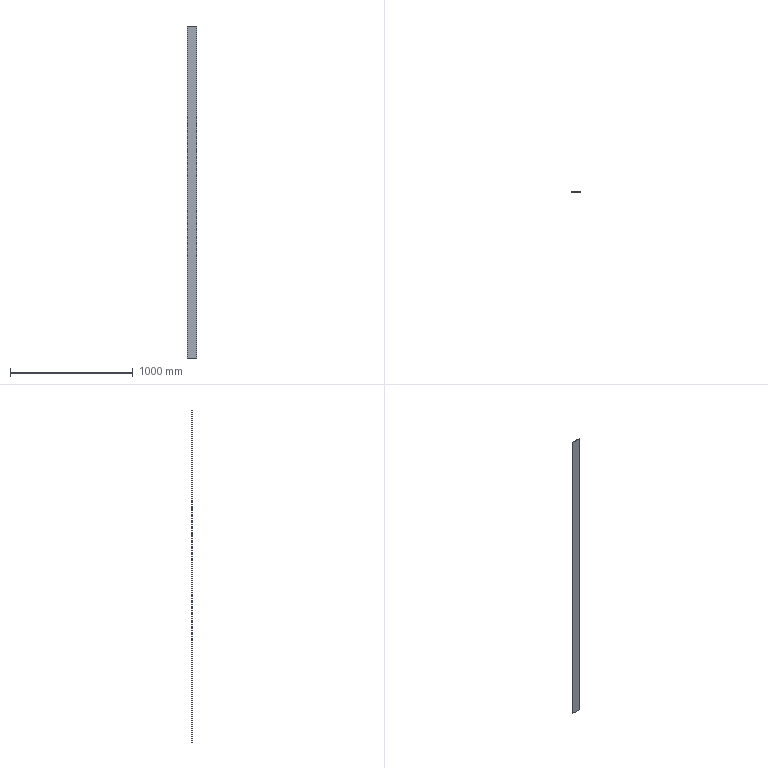Part | STEP file | Part6 | 1 solid | 6 faces | box 75 x 2 x 2700 mm | volume 405000 mm3 | plane 6
STEP:
#1=CARTESIAN_POINT('',(0.,0.,0.));
#2=DIRECTION('',(0.,0.,1.));
#3=DIRECTION('',(1.,0.,0.));
#4=AXIS2_PLACEMENT_3D('',#1,#2,#3);
#5=CARTESIAN_POINT('',(75.,0.,0.));
#6=VERTEX_POINT('',#5);
#7=CARTESIAN_POINT('',(75.,-2.,0.));
#8=VERTEX_POINT('',#7);
#9=CARTESIAN_POINT('',(75.,0.,0.));
#10=DIRECTION('',(0.,-1.,0.));
#11=VECTOR('',#10,1.);
#12=LINE('',#9,#11);
#13=CARTESIAN_POINT('',(75.,-2.,0.));
#14=DIRECTION('',(1.,0.,0.));
#15=DIRECTION('',(0.,1.,0.));
#16=AXIS2_PLACEMENT_3D('',#13,#14,#15);
#17=PLANE('',#16);
#18=CARTESIAN_POINT('',(2.,0.));
#19=DIRECTION('',(-1.,0.));
#20=VECTOR('',#19,1.);
#21=LINE('',#18,#20);
#22=(GEOMETRIC_REPRESENTATION_CONTEXT(2)PARAMETRIC_REPRESENTATION_CONTEXT()REPRESENTATION_CONTEXT('',''));
#23=DEFINITIONAL_REPRESENTATION('',(#21),#22);
#24=PCURVE('',#17,#23);
#25=CARTESIAN_POINT('',(37.5,-1.,0.));
#26=DIRECTION('',(0.,0.,1.));
#27=DIRECTION('',(1.,0.,0.));
#28=AXIS2_PLACEMENT_3D('',#25,#26,#27);
#29=PLANE('',#28);
#30=CARTESIAN_POINT('',(37.5,1.));
#31=DIRECTION('',(0.,-1.));
#32=VECTOR('',#31,1.);
#33=LINE('',#30,#32);
#34=(GEOMETRIC_REPRESENTATION_CONTEXT(2)PARAMETRIC_REPRESENTATION_CONTEXT()REPRESENTATION_CONTEXT('',''));
#35=DEFINITIONAL_REPRESENTATION('',(#33),#34);
#36=PCURVE('',#29,#35);
#37=SURFACE_CURVE('',#12,(#24,#36),.PCURVE_S1.);
#38=EDGE_CURVE('',#6,#8,#37,.T.);
#39=ORIENTED_EDGE('',*,*,#38,.F.);
#40=CARTESIAN_POINT('',(75.,0.,2700.));
#41=VERTEX_POINT('',#40);
#42=CARTESIAN_POINT('',(75.,0.,0.));
#43=DIRECTION('',(0.,0.,1.));
#44=VECTOR('',#43,1.);
#45=LINE('',#42,#44);
#46=CARTESIAN_POINT('',(2.,0.));
#47=DIRECTION('',(0.,1.));
#48=VECTOR('',#47,1.);
#49=LINE('',#46,#48);
#50=(GEOMETRIC_REPRESENTATION_CONTEXT(2)PARAMETRIC_REPRESENTATION_CONTEXT()REPRESENTATION_CONTEXT('',''));
#51=DEFINITIONAL_REPRESENTATION('',(#49),#50);
#52=PCURVE('',#17,#51);
#53=CARTESIAN_POINT('',(75.,0.,0.));
#54=DIRECTION('',(0.,1.,0.));
#55=DIRECTION('',(-1.,0.,0.));
#56=AXIS2_PLACEMENT_3D('',#53,#54,#55);
#57=PLANE('',#56);
#58=CARTESIAN_POINT('',(0.,0.));
#59=DIRECTION('',(0.,1.));
#60=VECTOR('',#59,1.);
#61=LINE('',#58,#60);
#62=(GEOMETRIC_REPRESENTATION_CONTEXT(2)PARAMETRIC_REPRESENTATION_CONTEXT()REPRESENTATION_CONTEXT('',''));
#63=DEFINITIONAL_REPRESENTATION('',(#61),#62);
#64=PCURVE('',#57,#63);
#65=SURFACE_CURVE('',#45,(#52,#64),.PCURVE_S1.);
#66=EDGE_CURVE('',#6,#41,#65,.T.);
#67=ORIENTED_EDGE('',*,*,#66,.T.);
#68=CARTESIAN_POINT('',(75.,-2.,2700.));
#69=VERTEX_POINT('',#68);
#70=CARTESIAN_POINT('',(75.,0.,2700.));
#71=DIRECTION('',(0.,1.,0.));
#72=VECTOR('',#71,1.);
#73=LINE('',#70,#72);
#74=CARTESIAN_POINT('',(2.,2700.));
#75=DIRECTION('',(1.,0.));
#76=VECTOR('',#75,1.);
#77=LINE('',#74,#76);
#78=(GEOMETRIC_REPRESENTATION_CONTEXT(2)PARAMETRIC_REPRESENTATION_CONTEXT()REPRESENTATION_CONTEXT('',''));
#79=DEFINITIONAL_REPRESENTATION('',(#77),#78);
#80=PCURVE('',#17,#79);
#81=CARTESIAN_POINT('',(37.5,-1.,2700.));
#82=DIRECTION('',(0.,0.,1.));
#83=DIRECTION('',(1.,0.,0.));
#84=AXIS2_PLACEMENT_3D('',#81,#82,#83);
#85=PLANE('',#84);
#86=CARTESIAN_POINT('',(37.5,1.));
#87=DIRECTION('',(0.,1.));
#88=VECTOR('',#87,1.);
#89=LINE('',#86,#88);
#90=(GEOMETRIC_REPRESENTATION_CONTEXT(2)PARAMETRIC_REPRESENTATION_CONTEXT()REPRESENTATION_CONTEXT('',''));
#91=DEFINITIONAL_REPRESENTATION('',(#89),#90);
#92=PCURVE('',#85,#91);
#93=SURFACE_CURVE('',#73,(#80,#92),.PCURVE_S1.);
#94=EDGE_CURVE('',#69,#41,#93,.T.);
#95=ORIENTED_EDGE('',*,*,#94,.F.);
#96=CARTESIAN_POINT('',(75.,-2.,0.));
#97=DIRECTION('',(0.,0.,1.));
#98=VECTOR('',#97,1.);
#99=LINE('',#96,#98);
#100=CARTESIAN_POINT('',(0.,0.));
#101=DIRECTION('',(0.,1.));
#102=VECTOR('',#101,1.);
#103=LINE('',#100,#102);
#104=(GEOMETRIC_REPRESENTATION_CONTEXT(2)PARAMETRIC_REPRESENTATION_CONTEXT()REPRESENTATION_CONTEXT('',''));
#105=DEFINITIONAL_REPRESENTATION('',(#103),#104);
#106=PCURVE('',#17,#105);
#107=CARTESIAN_POINT('',(0.,-2.,0.));
#108=DIRECTION('',(0.,-1.,0.));
#109=DIRECTION('',(1.,0.,0.));
#110=AXIS2_PLACEMENT_3D('',#107,#108,#109);
#111=PLANE('',#110);
#112=CARTESIAN_POINT('',(75.,0.));
#113=DIRECTION('',(0.,1.));
#114=VECTOR('',#113,1.);
#115=LINE('',#112,#114);
#116=(GEOMETRIC_REPRESENTATION_CONTEXT(2)PARAMETRIC_REPRESENTATION_CONTEXT()REPRESENTATION_CONTEXT('',''));
#117=DEFINITIONAL_REPRESENTATION('',(#115),#116);
#118=PCURVE('',#111,#117);
#119=SURFACE_CURVE('',#99,(#106,#118),.PCURVE_S1.);
#120=EDGE_CURVE('',#8,#69,#119,.T.);
#121=ORIENTED_EDGE('',*,*,#120,.F.);
#122=EDGE_LOOP('',(#39,#67,#95,#121));
#123=FACE_BOUND('',#122,.T.);
#124=ADVANCED_FACE('',(#123),#17,.T.);
#125=CARTESIAN_POINT('',(0.,-2.,0.));
#126=VERTEX_POINT('',#125);
#127=CARTESIAN_POINT('',(75.,-2.,0.));
#128=DIRECTION('',(-1.,0.,0.));
#129=VECTOR('',#128,1.);
#130=LINE('',#127,#129);
#131=CARTESIAN_POINT('',(75.,0.));
#132=DIRECTION('',(-1.,0.));
#133=VECTOR('',#132,1.);
#134=LINE('',#131,#133);
#135=(GEOMETRIC_REPRESENTATION_CONTEXT(2)PARAMETRIC_REPRESENTATION_CONTEXT()REPRESENTATION_CONTEXT('',''));
#136=DEFINITIONAL_REPRESENTATION('',(#134),#135);
#137=PCURVE('',#111,#136);
#138=CARTESIAN_POINT('',(37.5,-1.));
#139=DIRECTION('',(-1.,0.));
#140=VECTOR('',#139,1.);
#141=LINE('',#138,#140);
#142=(GEOMETRIC_REPRESENTATION_CONTEXT(2)PARAMETRIC_REPRESENTATION_CONTEXT()REPRESENTATION_CONTEXT('',''));
#143=DEFINITIONAL_REPRESENTATION('',(#141),#142);
#144=PCURVE('',#29,#143);
#145=SURFACE_CURVE('',#130,(#137,#144),.PCURVE_S1.);
#146=EDGE_CURVE('',#8,#126,#145,.T.);
#147=ORIENTED_EDGE('',*,*,#146,.F.);
#148=ORIENTED_EDGE('',*,*,#120,.T.);
#149=CARTESIAN_POINT('',(0.,-2.,2700.));
#150=VERTEX_POINT('',#149);
#151=CARTESIAN_POINT('',(75.,-2.,2700.));
#152=DIRECTION('',(1.,0.,0.));
#153=VECTOR('',#152,1.);
#154=LINE('',#151,#153);
#155=CARTESIAN_POINT('',(75.,2700.));
#156=DIRECTION('',(1.,0.));
#157=VECTOR('',#156,1.);
#158=LINE('',#155,#157);
#159=(GEOMETRIC_REPRESENTATION_CONTEXT(2)PARAMETRIC_REPRESENTATION_CONTEXT()REPRESENTATION_CONTEXT('',''));
#160=DEFINITIONAL_REPRESENTATION('',(#158),#159);
#161=PCURVE('',#111,#160);
#162=CARTESIAN_POINT('',(37.5,-1.));
#163=DIRECTION('',(1.,0.));
#164=VECTOR('',#163,1.);
#165=LINE('',#162,#164);
#166=(GEOMETRIC_REPRESENTATION_CONTEXT(2)PARAMETRIC_REPRESENTATION_CONTEXT()REPRESENTATION_CONTEXT('',''));
#167=DEFINITIONAL_REPRESENTATION('',(#165),#166);
#168=PCURVE('',#85,#167);
#169=SURFACE_CURVE('',#154,(#161,#168),.PCURVE_S1.);
#170=EDGE_CURVE('',#150,#69,#169,.T.);
#171=ORIENTED_EDGE('',*,*,#170,.F.);
#172=CARTESIAN_POINT('',(0.,-2.,0.));
#173=DIRECTION('',(0.,0.,1.));
#174=VECTOR('',#173,1.);
#175=LINE('',#172,#174);
#176=CARTESIAN_POINT('',(0.,0.));
#177=DIRECTION('',(0.,1.));
#178=VECTOR('',#177,1.);
#179=LINE('',#176,#178);
#180=(GEOMETRIC_REPRESENTATION_CONTEXT(2)PARAMETRIC_REPRESENTATION_CONTEXT()REPRESENTATION_CONTEXT('',''));
#181=DEFINITIONAL_REPRESENTATION('',(#179),#180);
#182=PCURVE('',#111,#181);
#183=CARTESIAN_POINT('',(0.,0.,0.));
#184=DIRECTION('',(-1.,0.,0.));
#185=DIRECTION('',(0.,-1.,0.));
#186=AXIS2_PLACEMENT_3D('',#183,#184,#185);
#187=PLANE('',#186);
#188=CARTESIAN_POINT('',(2.,0.));
#189=DIRECTION('',(0.,1.));
#190=VECTOR('',#189,1.);
#191=LINE('',#188,#190);
#192=(GEOMETRIC_REPRESENTATION_CONTEXT(2)PARAMETRIC_REPRESENTATION_CONTEXT()REPRESENTATION_CONTEXT('',''));
#193=DEFINITIONAL_REPRESENTATION('',(#191),#192);
#194=PCURVE('',#187,#193);
#195=SURFACE_CURVE('',#175,(#182,#194),.PCURVE_S1.);
#196=EDGE_CURVE('',#126,#150,#195,.T.);
#197=ORIENTED_EDGE('',*,*,#196,.F.);
#198=EDGE_LOOP('',(#147,#148,#171,#197));
#199=FACE_BOUND('',#198,.T.);
#200=ADVANCED_FACE('',(#199),#111,.T.);
#201=CARTESIAN_POINT('',(0.,0.,0.));
#202=VERTEX_POINT('',#201);
#203=CARTESIAN_POINT('',(0.,-2.,0.));
#204=DIRECTION('',(0.,1.,0.));
#205=VECTOR('',#204,1.);
#206=LINE('',#203,#205);
#207=CARTESIAN_POINT('',(2.,0.));
#208=DIRECTION('',(-1.,0.));
#209=VECTOR('',#208,1.);
#210=LINE('',#207,#209);
#211=(GEOMETRIC_REPRESENTATION_CONTEXT(2)PARAMETRIC_REPRESENTATION_CONTEXT()REPRESENTATION_CONTEXT('',''));
#212=DEFINITIONAL_REPRESENTATION('',(#210),#211);
#213=PCURVE('',#187,#212);
#214=CARTESIAN_POINT('',(-37.5,-1.));
#215=DIRECTION('',(0.,1.));
#216=VECTOR('',#215,1.);
#217=LINE('',#214,#216);
#218=(GEOMETRIC_REPRESENTATION_CONTEXT(2)PARAMETRIC_REPRESENTATION_CONTEXT()REPRESENTATION_CONTEXT('',''));
#219=DEFINITIONAL_REPRESENTATION('',(#217),#218);
#220=PCURVE('',#29,#219);
#221=SURFACE_CURVE('',#206,(#213,#220),.PCURVE_S1.);
#222=EDGE_CURVE('',#126,#202,#221,.T.);
#223=ORIENTED_EDGE('',*,*,#222,.F.);
#224=ORIENTED_EDGE('',*,*,#196,.T.);
#225=CARTESIAN_POINT('',(0.,0.,2700.));
#226=VERTEX_POINT('',#225);
#227=CARTESIAN_POINT('',(0.,-2.,2700.));
#228=DIRECTION('',(0.,-1.,0.));
#229=VECTOR('',#228,1.);
#230=LINE('',#227,#229);
#231=CARTESIAN_POINT('',(2.,2700.));
#232=DIRECTION('',(1.,0.));
#233=VECTOR('',#232,1.);
#234=LINE('',#231,#233);
#235=(GEOMETRIC_REPRESENTATION_CONTEXT(2)PARAMETRIC_REPRESENTATION_CONTEXT()REPRESENTATION_CONTEXT('',''));
#236=DEFINITIONAL_REPRESENTATION('',(#234),#235);
#237=PCURVE('',#187,#236);
#238=CARTESIAN_POINT('',(-37.5,-1.));
#239=DIRECTION('',(0.,-1.));
#240=VECTOR('',#239,1.);
#241=LINE('',#238,#240);
#242=(GEOMETRIC_REPRESENTATION_CONTEXT(2)PARAMETRIC_REPRESENTATION_CONTEXT()REPRESENTATION_CONTEXT('',''));
#243=DEFINITIONAL_REPRESENTATION('',(#241),#242);
#244=PCURVE('',#85,#243);
#245=SURFACE_CURVE('',#230,(#237,#244),.PCURVE_S1.);
#246=EDGE_CURVE('',#226,#150,#245,.T.);
#247=ORIENTED_EDGE('',*,*,#246,.F.);
#248=CARTESIAN_POINT('',(0.,0.,0.));
#249=DIRECTION('',(0.,0.,1.));
#250=VECTOR('',#249,1.);
#251=LINE('',#248,#250);
#252=CARTESIAN_POINT('',(0.,0.));
#253=DIRECTION('',(0.,1.));
#254=VECTOR('',#253,1.);
#255=LINE('',#252,#254);
#256=(GEOMETRIC_REPRESENTATION_CONTEXT(2)PARAMETRIC_REPRESENTATION_CONTEXT()REPRESENTATION_CONTEXT('',''));
#257=DEFINITIONAL_REPRESENTATION('',(#255),#256);
#258=PCURVE('',#187,#257);
#259=CARTESIAN_POINT('',(75.,0.));
#260=DIRECTION('',(0.,1.));
#261=VECTOR('',#260,1.);
#262=LINE('',#259,#261);
#263=(GEOMETRIC_REPRESENTATION_CONTEXT(2)PARAMETRIC_REPRESENTATION_CONTEXT()REPRESENTATION_CONTEXT('',''));
#264=DEFINITIONAL_REPRESENTATION('',(#262),#263);
#265=PCURVE('',#57,#264);
#266=SURFACE_CURVE('',#251,(#258,#265),.PCURVE_S1.);
#267=EDGE_CURVE('',#202,#226,#266,.T.);
#268=ORIENTED_EDGE('',*,*,#267,.F.);
#269=EDGE_LOOP('',(#223,#224,#247,#268));
#270=FACE_BOUND('',#269,.T.);
#271=ADVANCED_FACE('',(#270),#187,.T.);
#272=CARTESIAN_POINT('',(0.,0.,0.));
#273=DIRECTION('',(1.,0.,0.));
#274=VECTOR('',#273,1.);
#275=LINE('',#272,#274);
#276=CARTESIAN_POINT('',(75.,0.));
#277=DIRECTION('',(-1.,0.));
#278=VECTOR('',#277,1.);
#279=LINE('',#276,#278);
#280=(GEOMETRIC_REPRESENTATION_CONTEXT(2)PARAMETRIC_REPRESENTATION_CONTEXT()REPRESENTATION_CONTEXT('',''));
#281=DEFINITIONAL_REPRESENTATION('',(#279),#280);
#282=PCURVE('',#57,#281);
#283=CARTESIAN_POINT('',(-37.5,1.));
#284=DIRECTION('',(1.,0.));
#285=VECTOR('',#284,1.);
#286=LINE('',#283,#285);
#287=(GEOMETRIC_REPRESENTATION_CONTEXT(2)PARAMETRIC_REPRESENTATION_CONTEXT()REPRESENTATION_CONTEXT('',''));
#288=DEFINITIONAL_REPRESENTATION('',(#286),#287);
#289=PCURVE('',#29,#288);
#290=SURFACE_CURVE('',#275,(#282,#289),.PCURVE_S1.);
#291=EDGE_CURVE('',#202,#6,#290,.T.);
#292=ORIENTED_EDGE('',*,*,#291,.F.);
#293=ORIENTED_EDGE('',*,*,#267,.T.);
#294=CARTESIAN_POINT('',(0.,0.,2700.));
#295=DIRECTION('',(-1.,0.,0.));
#296=VECTOR('',#295,1.);
#297=LINE('',#294,#296);
#298=CARTESIAN_POINT('',(75.,2700.));
#299=DIRECTION('',(1.,0.));
#300=VECTOR('',#299,1.);
#301=LINE('',#298,#300);
#302=(GEOMETRIC_REPRESENTATION_CONTEXT(2)PARAMETRIC_REPRESENTATION_CONTEXT()REPRESENTATION_CONTEXT('',''));
#303=DEFINITIONAL_REPRESENTATION('',(#301),#302);
#304=PCURVE('',#57,#303);
#305=CARTESIAN_POINT('',(-37.5,1.));
#306=DIRECTION('',(-1.,0.));
#307=VECTOR('',#306,1.);
#308=LINE('',#305,#307);
#309=(GEOMETRIC_REPRESENTATION_CONTEXT(2)PARAMETRIC_REPRESENTATION_CONTEXT()REPRESENTATION_CONTEXT('',''));
#310=DEFINITIONAL_REPRESENTATION('',(#308),#309);
#311=PCURVE('',#85,#310);
#312=SURFACE_CURVE('',#297,(#304,#311),.PCURVE_S1.);
#313=EDGE_CURVE('',#41,#226,#312,.T.);
#314=ORIENTED_EDGE('',*,*,#313,.F.);
#315=ORIENTED_EDGE('',*,*,#66,.F.);
#316=EDGE_LOOP('',(#292,#293,#314,#315));
#317=FACE_BOUND('',#316,.T.);
#318=ADVANCED_FACE('',(#317),#57,.T.);
#319=ORIENTED_EDGE('',*,*,#291,.T.);
#320=ORIENTED_EDGE('',*,*,#38,.T.);
#321=ORIENTED_EDGE('',*,*,#146,.T.);
#322=ORIENTED_EDGE('',*,*,#222,.T.);
#323=EDGE_LOOP('',(#319,#320,#321,#322));
#324=FACE_BOUND('',#323,.T.);
#325=ADVANCED_FACE('',(#324),#29,.F.);
#326=ORIENTED_EDGE('',*,*,#313,.T.);
#327=ORIENTED_EDGE('',*,*,#246,.T.);
#328=ORIENTED_EDGE('',*,*,#170,.T.);
#329=ORIENTED_EDGE('',*,*,#94,.T.);
#330=EDGE_LOOP('',(#326,#327,#328,#329));
#331=FACE_BOUND('',#330,.T.);
#332=ADVANCED_FACE('',(#331),#85,.T.);
#333=CLOSED_SHELL('',(#124,#200,#271,#318,#325,#332));
#334=MANIFOLD_SOLID_BREP('',#333);
#335=(LENGTH_UNIT()NAMED_UNIT(*)SI_UNIT(.MILLI.,.METRE.));
#336=UNCERTAINTY_MEASURE_WITH_UNIT(LENGTH_MEASURE(0.0000001),#335,'','');
#337=(NAMED_UNIT(*)PLANE_ANGLE_UNIT()SI_UNIT($,.RADIAN.));
#338=(NAMED_UNIT(*)SI_UNIT($,.STERADIAN.)SOLID_ANGLE_UNIT());
#339=(GEOMETRIC_REPRESENTATION_CONTEXT(3)GLOBAL_UNCERTAINTY_ASSIGNED_CONTEXT((#336))GLOBAL_UNIT_ASSIGNED_CONTEXT((#335,#337,#338))REPRESENTATION_CONTEXT('',''));
#340=ADVANCED_BREP_SHAPE_REPRESENTATION('',(#4,#334),#339);